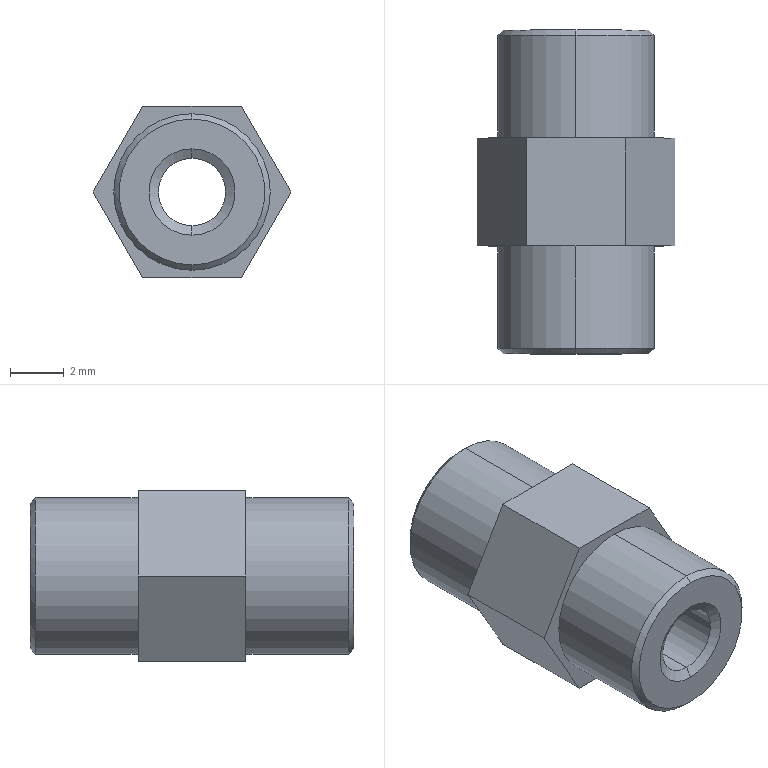Part | STEP file | 6022D044 | 1 solid | 24 faces | box 7.332 x 12 x 6.35 mm | volume 290.823 mm3 | plane 10 | cone 8 | cylinder 6 | commonest cylinder face diameters 5.8 x4 2.5 x2